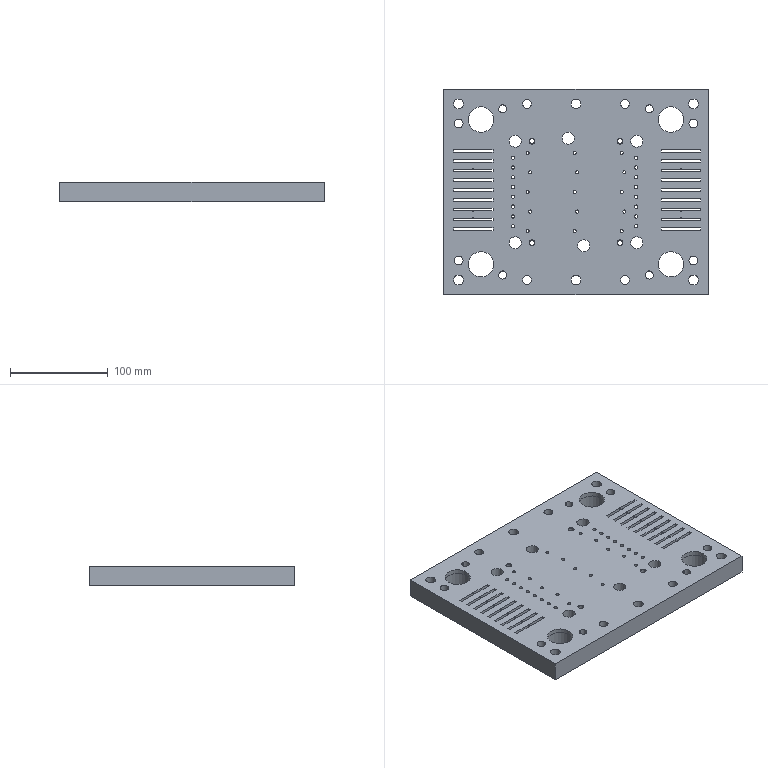Part | STEP file | 1 solid | 260 faces | box 270 x 210 x 20 mm | volume 990769 mm3 | plane 126 | cylinder 123 | cone 11 | commonest cylinder face diameters 3.1 x36 3.5 x16 3.2 x15 1 x12 9 x8 14 x8